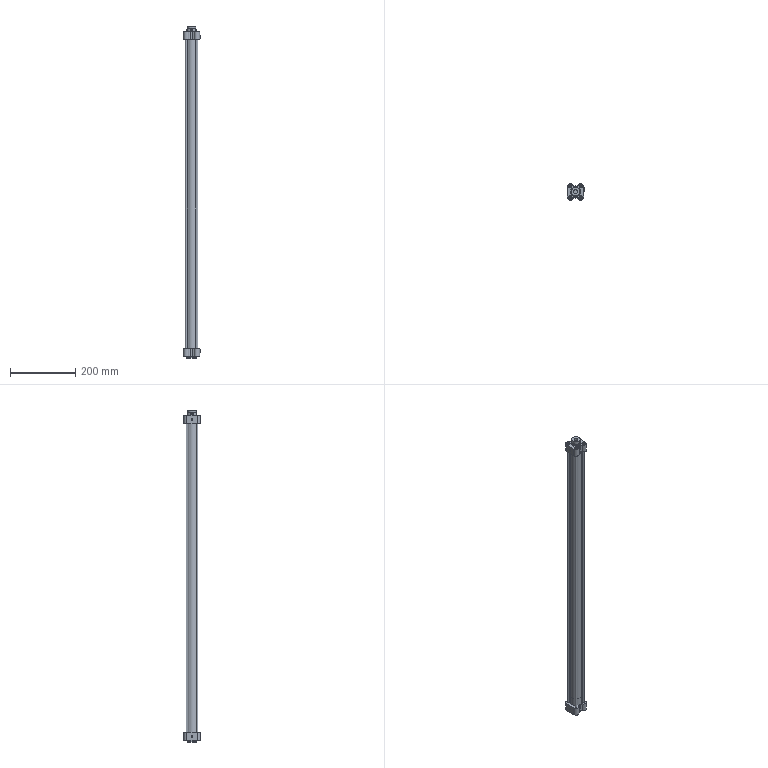Part | STEP file | 160884 CRDNG-32-900-PPV-A---(ZR) | 1 solid | 177 faces | box 53 x 50 x 1014 mm | volume 321289 mm3 | plane 91 | cylinder 58 | cone 23 | torus 5 | commonest cylinder face diameters 4.917 x10 10 x10 17.4 x8 6 x4 9 x4 9.4 x4